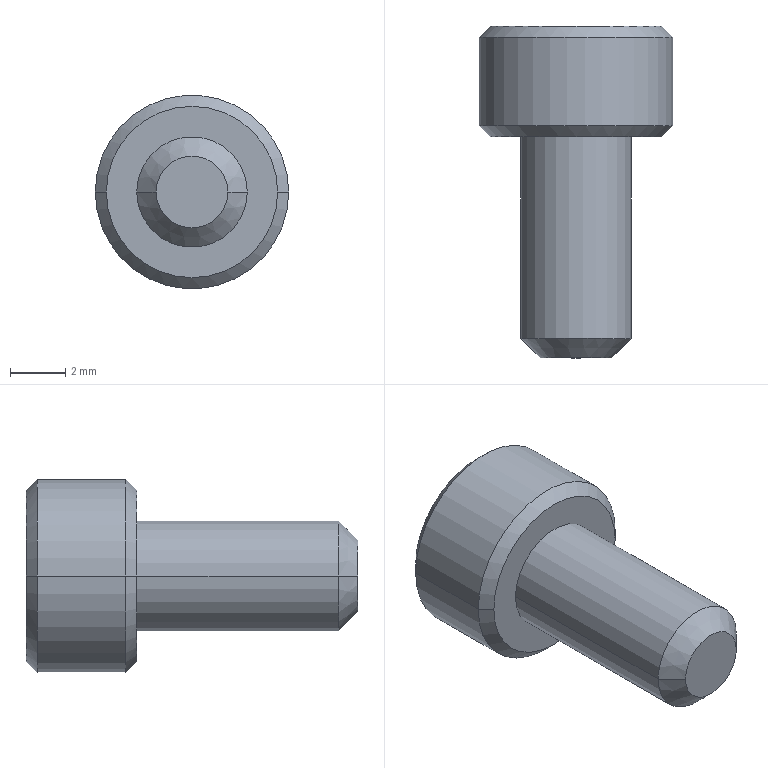Part | STEP file | BB62-M4-8L-1 | 1 solid | 27 faces | box 7 x 12 x 7 mm | volume 229.916 mm3 | plane 15 | cone 8 | cylinder 4 | commonest cylinder face diameters 4 x2 7 x2
STEP:
#1=CARTESIAN_POINT('',(0.,1.007,0.));
#2=VERTEX_POINT('',#1);
#3=CARTESIAN_POINT('',(1.72,2.,0.));
#4=VERTEX_POINT('',#3);
#5=CARTESIAN_POINT('',(0.,1.007,0.));
#6=DIRECTION('',(0.866,0.5,0.));
#7=VECTOR('',#6,1000.);
#8=LINE('',#5,#7);
#9=EDGE_CURVE('',#2,#4,#8,.T.);
#10=ORIENTED_EDGE('',*,*,#9,.F.);
#11=CARTESIAN_POINT('',(-1.72,2.,0.));
#12=VERTEX_POINT('',#11);
#13=CARTESIAN_POINT('',(0.,1.007,0.));
#14=DIRECTION('',(-0.866,0.5,0.));
#15=VECTOR('',#14,1000.);
#16=LINE('',#13,#15);
#17=EDGE_CURVE('',#2,#12,#16,.T.);
#18=ORIENTED_EDGE('',*,*,#17,.T.);
#19=CARTESIAN_POINT('',(-1.49,2.,0.86));
#20=VERTEX_POINT('',#19);
#21=CARTESIAN_POINT('',(0.,2.,0.));
#22=DIRECTION('',(0.,-1.,0.));
#23=DIRECTION('',(-1.,0.,0.));
#24=AXIS2_PLACEMENT_3D('',#21,#22,#23);
#25=CIRCLE('',#24,1.72);
#26=EDGE_CURVE('',#20,#12,#25,.T.);
#27=ORIENTED_EDGE('',*,*,#26,.F.);
#28=CARTESIAN_POINT('',(0.,2.,1.72));
#29=VERTEX_POINT('',#28);
#30=CARTESIAN_POINT('',(0.,2.,0.));
#31=DIRECTION('',(0.,-1.,0.));
#32=DIRECTION('',(-1.,0.,0.));
#33=AXIS2_PLACEMENT_3D('',#30,#31,#32);
#34=CIRCLE('',#33,1.72);
#35=EDGE_CURVE('',#29,#20,#34,.T.);
#36=ORIENTED_EDGE('',*,*,#35,.F.);
#37=CARTESIAN_POINT('',(1.49,2.,0.86));
#38=VERTEX_POINT('',#37);
#39=CARTESIAN_POINT('',(0.,2.,0.));
#40=DIRECTION('',(0.,-1.,0.));
#41=DIRECTION('',(-1.,0.,0.));
#42=AXIS2_PLACEMENT_3D('',#39,#40,#41);
#43=CIRCLE('',#42,1.72);
#44=EDGE_CURVE('',#38,#29,#43,.T.);
#45=ORIENTED_EDGE('',*,*,#44,.F.);
#46=CARTESIAN_POINT('',(0.,2.,0.));
#47=DIRECTION('',(0.,-1.,0.));
#48=DIRECTION('',(-1.,0.,0.));
#49=AXIS2_PLACEMENT_3D('',#46,#47,#48);
#50=CIRCLE('',#49,1.72);
#51=EDGE_CURVE('',#4,#38,#50,.T.);
#52=ORIENTED_EDGE('',*,*,#51,.F.);
#53=EDGE_LOOP('',(#10,#18,#27,#36,#45,#52));
#54=FACE_OUTER_BOUND('',#53,.T.);
#55=CARTESIAN_POINT('',(0.,1001.007,0.));
#56=DIRECTION('',(0.,1.,0.));
#57=DIRECTION('',(1.,0.,0.));
#58=AXIS2_PLACEMENT_3D('',#55,#56,#57);
#59=CONICAL_SURFACE('',#58,1732.051,1.047);
#60=ADVANCED_FACE('',(#54),#59,.F.);
#61=CARTESIAN_POINT('',(1.3,-8.,0.));
#62=VERTEX_POINT('',#61);
#63=CARTESIAN_POINT('',(-1.3,-8.,0.));
#64=VERTEX_POINT('',#63);
#65=CARTESIAN_POINT('',(0.,-8.,0.));
#66=DIRECTION('',(0.,1.,0.));
#67=DIRECTION('',(1.,0.,0.));
#68=AXIS2_PLACEMENT_3D('',#65,#66,#67);
#69=CIRCLE('',#68,1.3);
#70=EDGE_CURVE('',#62,#64,#69,.T.);
#71=ORIENTED_EDGE('',*,*,#70,.T.);
#72=CARTESIAN_POINT('',(-2.,-7.3,0.));
#73=VERTEX_POINT('',#72);
#74=CARTESIAN_POINT('',(-1.3,-8.,0.));
#75=DIRECTION('',(-0.7071,0.7071,0.));
#76=VECTOR('',#75,1000.);
#77=LINE('',#74,#76);
#78=EDGE_CURVE('',#64,#73,#77,.T.);
#79=ORIENTED_EDGE('',*,*,#78,.T.);
#80=CARTESIAN_POINT('',(2.,-7.3,0.));
#81=VERTEX_POINT('',#80);
#82=CARTESIAN_POINT('',(0.,-7.3,0.));
#83=DIRECTION('',(0.,-1.,0.));
#84=DIRECTION('',(-1.,0.,0.));
#85=AXIS2_PLACEMENT_3D('',#82,#83,#84);
#86=CIRCLE('',#85,2.);
#87=EDGE_CURVE('',#73,#81,#86,.T.);
#88=ORIENTED_EDGE('',*,*,#87,.T.);
#89=CARTESIAN_POINT('',(1.3,-8.,0.));
#90=DIRECTION('',(0.7071,0.7071,0.));
#91=VECTOR('',#90,1000.);
#92=LINE('',#89,#91);
#93=EDGE_CURVE('',#62,#81,#92,.T.);
#94=ORIENTED_EDGE('',*,*,#93,.F.);
#95=EDGE_LOOP('',(#71,#79,#88,#94));
#96=FACE_OUTER_BOUND('',#95,.T.);
#97=CARTESIAN_POINT('',(0.,-8.,0.));
#98=DIRECTION('',(0.,1.,0.));
#99=DIRECTION('',(1.,0.,0.));
#100=AXIS2_PLACEMENT_3D('',#97,#98,#99);
#101=CONICAL_SURFACE('',#100,1.3,0.7854);
#102=ADVANCED_FACE('',(#96),#101,.T.);
#103=ORIENTED_EDGE('',*,*,#87,.F.);
#104=CARTESIAN_POINT('',(-2.,0.,0.));
#105=VERTEX_POINT('',#104);
#106=CARTESIAN_POINT('',(-2.,-7.3,0.));
#107=DIRECTION('',(0.,1.,0.));
#108=VECTOR('',#107,1000.);
#109=LINE('',#106,#108);
#110=EDGE_CURVE('',#73,#105,#109,.T.);
#111=ORIENTED_EDGE('',*,*,#110,.T.);
#112=CARTESIAN_POINT('',(2.,0.,0.));
#113=VERTEX_POINT('',#112);
#114=CARTESIAN_POINT('',(0.,0.,0.));
#115=DIRECTION('',(0.,-1.,0.));
#116=DIRECTION('',(-1.,0.,0.));
#117=AXIS2_PLACEMENT_3D('',#114,#115,#116);
#118=CIRCLE('',#117,2.);
#119=EDGE_CURVE('',#105,#113,#118,.T.);
#120=ORIENTED_EDGE('',*,*,#119,.T.);
#121=CARTESIAN_POINT('',(2.,-7.3,0.));
#122=DIRECTION('',(0.,1.,0.));
#123=VECTOR('',#122,1000.);
#124=LINE('',#121,#123);
#125=EDGE_CURVE('',#81,#113,#124,.T.);
#126=ORIENTED_EDGE('',*,*,#125,.F.);
#127=EDGE_LOOP('',(#103,#111,#120,#126));
#128=FACE_OUTER_BOUND('',#127,.T.);
#129=CARTESIAN_POINT('',(0.,-7.3,0.));
#130=DIRECTION('',(0.,1.,0.));
#131=DIRECTION('',(1.,0.,0.));
#132=AXIS2_PLACEMENT_3D('',#129,#130,#131);
#133=CYLINDRICAL_SURFACE('',#132,2.);
#134=ADVANCED_FACE('',(#128),#133,.T.);
#135=CARTESIAN_POINT('',(-3.1,4.,0.));
#136=VERTEX_POINT('',#135);
#137=CARTESIAN_POINT('',(3.1,4.,0.));
#138=VERTEX_POINT('',#137);
#139=CARTESIAN_POINT('',(0.,4.,0.));
#140=DIRECTION('',(0.,-1.,0.));
#141=DIRECTION('',(-1.,0.,0.));
#142=AXIS2_PLACEMENT_3D('',#139,#140,#141);
#143=CIRCLE('',#142,3.1);
#144=EDGE_CURVE('',#136,#138,#143,.T.);
#145=ORIENTED_EDGE('',*,*,#144,.T.);
#146=CARTESIAN_POINT('',(3.5,3.6,0.));
#147=VERTEX_POINT('',#146);
#148=CARTESIAN_POINT('',(3.5,3.6,0.));
#149=DIRECTION('',(0.7071,-0.7071,0.));
#150=VECTOR('',#149,1000.);
#151=LINE('',#148,#150);
#152=EDGE_CURVE('',#138,#147,#151,.T.);
#153=ORIENTED_EDGE('',*,*,#152,.T.);
#154=CARTESIAN_POINT('',(-3.5,3.6,0.));
#155=VERTEX_POINT('',#154);
#156=CARTESIAN_POINT('',(0.,3.6,0.));
#157=DIRECTION('',(0.,-1.,0.));
#158=DIRECTION('',(-1.,0.,0.));
#159=AXIS2_PLACEMENT_3D('',#156,#157,#158);
#160=CIRCLE('',#159,3.5);
#161=EDGE_CURVE('',#155,#147,#160,.T.);
#162=ORIENTED_EDGE('',*,*,#161,.F.);
#163=CARTESIAN_POINT('',(-3.5,3.6,0.));
#164=DIRECTION('',(-0.7071,-0.7071,0.));
#165=VECTOR('',#164,1000.);
#166=LINE('',#163,#165);
#167=EDGE_CURVE('',#136,#155,#166,.T.);
#168=ORIENTED_EDGE('',*,*,#167,.F.);
#169=EDGE_LOOP('',(#145,#153,#162,#168));
#170=FACE_OUTER_BOUND('',#169,.T.);
#171=CARTESIAN_POINT('',(0.,3.6,0.));
#172=DIRECTION('',(0.,-1.,0.));
#173=DIRECTION('',(-1.,0.,0.));
#174=AXIS2_PLACEMENT_3D('',#171,#172,#173);
#175=CONICAL_SURFACE('',#174,3.5,0.7854);
#176=ADVANCED_FACE('',(#170),#175,.T.);
#177=ORIENTED_EDGE('',*,*,#161,.T.);
#178=CARTESIAN_POINT('',(3.5,0.4,0.));
#179=VERTEX_POINT('',#178);
#180=CARTESIAN_POINT('',(3.5,1.62,0.));
#181=DIRECTION('',(0.,-1.,0.));
#182=VECTOR('',#181,1000.);
#183=LINE('',#180,#182);
#184=EDGE_CURVE('',#147,#179,#183,.T.);
#185=ORIENTED_EDGE('',*,*,#184,.T.);
#186=CARTESIAN_POINT('',(-3.5,0.4,0.));
#187=VERTEX_POINT('',#186);
#188=CARTESIAN_POINT('',(0.,0.4,0.));
#189=DIRECTION('',(0.,-1.,0.));
#190=DIRECTION('',(-1.,0.,0.));
#191=AXIS2_PLACEMENT_3D('',#188,#189,#190);
#192=CIRCLE('',#191,3.5);
#193=EDGE_CURVE('',#187,#179,#192,.T.);
#194=ORIENTED_EDGE('',*,*,#193,.F.);
#195=CARTESIAN_POINT('',(-3.5,1.62,0.));
#196=DIRECTION('',(0.,-1.,0.));
#197=VECTOR('',#196,1000.);
#198=LINE('',#195,#197);
#199=EDGE_CURVE('',#155,#187,#198,.T.);
#200=ORIENTED_EDGE('',*,*,#199,.F.);
#201=EDGE_LOOP('',(#177,#185,#194,#200));
#202=FACE_OUTER_BOUND('',#201,.T.);
#203=CARTESIAN_POINT('',(0.,1.62,0.));
#204=DIRECTION('',(0.,-1.,0.));
#205=DIRECTION('',(-1.,0.,0.));
#206=AXIS2_PLACEMENT_3D('',#203,#204,#205);
#207=CYLINDRICAL_SURFACE('',#206,3.5);
#208=ADVANCED_FACE('',(#202),#207,.T.);
#209=CARTESIAN_POINT('',(-3.1,0.,0.));
#210=VERTEX_POINT('',#209);
#211=CARTESIAN_POINT('',(3.1,0.,0.));
#212=VERTEX_POINT('',#211);
#213=CARTESIAN_POINT('',(0.,0.,0.));
#214=DIRECTION('',(0.,-1.,0.));
#215=DIRECTION('',(-1.,0.,0.));
#216=AXIS2_PLACEMENT_3D('',#213,#214,#215);
#217=CIRCLE('',#216,3.1);
#218=EDGE_CURVE('',#210,#212,#217,.T.);
#219=ORIENTED_EDGE('',*,*,#218,.F.);
#220=CARTESIAN_POINT('',(-3.1,0.,0.));
#221=DIRECTION('',(-0.7071,0.7071,0.));
#222=VECTOR('',#221,1000.);
#223=LINE('',#220,#222);
#224=EDGE_CURVE('',#210,#187,#223,.T.);
#225=ORIENTED_EDGE('',*,*,#224,.T.);
#226=ORIENTED_EDGE('',*,*,#193,.T.);
#227=CARTESIAN_POINT('',(3.1,0.,0.));
#228=DIRECTION('',(0.7071,0.7071,0.));
#229=VECTOR('',#228,1000.);
#230=LINE('',#227,#229);
#231=EDGE_CURVE('',#212,#179,#230,.T.);
#232=ORIENTED_EDGE('',*,*,#231,.F.);
#233=EDGE_LOOP('',(#219,#225,#226,#232));
#234=FACE_OUTER_BOUND('',#233,.T.);
#235=CARTESIAN_POINT('',(0.,0.,0.));
#236=DIRECTION('',(0.,1.,0.));
#237=DIRECTION('',(1.,0.,0.));
#238=AXIS2_PLACEMENT_3D('',#235,#236,#237);
#239=CONICAL_SURFACE('',#238,3.1,0.7854);
#240=ADVANCED_FACE('',(#234),#239,.T.);
#241=ORIENTED_EDGE('',*,*,#144,.F.);
#242=CARTESIAN_POINT('',(0.,4.,0.));
#243=DIRECTION('',(0.,-1.,0.));
#244=DIRECTION('',(-1.,0.,0.));
#245=AXIS2_PLACEMENT_3D('',#242,#243,#244);
#246=CIRCLE('',#245,3.1);
#247=EDGE_CURVE('',#138,#136,#246,.T.);
#248=ORIENTED_EDGE('',*,*,#247,.F.);
#249=EDGE_LOOP('',(#241,#248));
#250=FACE_OUTER_BOUND('',#249,.T.);
#251=CARTESIAN_POINT('',(0.,4.,-1.72));
#252=VERTEX_POINT('',#251);
#253=CARTESIAN_POINT('',(-1.49,4.,-0.86));
#254=VERTEX_POINT('',#253);
#255=CARTESIAN_POINT('',(0.,4.,-1.72));
#256=DIRECTION('',(-0.866,0.,0.5));
#257=VECTOR('',#256,1000.);
#258=LINE('',#255,#257);
#259=EDGE_CURVE('',#252,#254,#258,.T.);
#260=ORIENTED_EDGE('',*,*,#259,.F.);
#261=CARTESIAN_POINT('',(1.49,4.,-0.86));
#262=VERTEX_POINT('',#261);
#263=CARTESIAN_POINT('',(1.49,4.,-0.86));
#264=DIRECTION('',(-0.866,0.,-0.5));
#265=VECTOR('',#264,1000.);
#266=LINE('',#263,#265);
#267=EDGE_CURVE('',#262,#252,#266,.T.);
#268=ORIENTED_EDGE('',*,*,#267,.F.);
#269=CARTESIAN_POINT('',(1.49,4.,0.86));
#270=VERTEX_POINT('',#269);
#271=CARTESIAN_POINT('',(1.49,4.,0.86));
#272=DIRECTION('',(0.,0.,-1.));
#273=VECTOR('',#272,1000.);
#274=LINE('',#271,#273);
#275=EDGE_CURVE('',#270,#262,#274,.T.);
#276=ORIENTED_EDGE('',*,*,#275,.F.);
#277=CARTESIAN_POINT('',(0.,4.,1.72));
#278=VERTEX_POINT('',#277);
#279=CARTESIAN_POINT('',(0.,4.,1.72));
#280=DIRECTION('',(0.866,0.,-0.5));
#281=VECTOR('',#280,1000.);
#282=LINE('',#279,#281);
#283=EDGE_CURVE('',#278,#270,#282,.T.);
#284=ORIENTED_EDGE('',*,*,#283,.F.);
#285=CARTESIAN_POINT('',(-1.49,4.,0.86));
#286=VERTEX_POINT('',#285);
#287=CARTESIAN_POINT('',(-1.49,4.,0.86));
#288=DIRECTION('',(0.866,0.,0.5));
#289=VECTOR('',#288,1000.);
#290=LINE('',#287,#289);
#291=EDGE_CURVE('',#286,#278,#290,.T.);
#292=ORIENTED_EDGE('',*,*,#291,.F.);
#293=CARTESIAN_POINT('',(-1.49,4.,-0.86));
#294=DIRECTION('',(0.,0.,1.));
#295=VECTOR('',#294,1000.);
#296=LINE('',#293,#295);
#297=EDGE_CURVE('',#254,#286,#296,.T.);
#298=ORIENTED_EDGE('',*,*,#297,.F.);
#299=EDGE_LOOP('',(#260,#268,#276,#284,#292,#298));
#300=FACE_BOUND('',#299,.T.);
#301=CARTESIAN_POINT('',(3.1,4.,0.));
#302=DIRECTION('',(0.,1.,0.));
#303=DIRECTION('',(1.,0.,0.));
#304=AXIS2_PLACEMENT_3D('',#301,#302,#303);
#305=PLANE('',#304);
#306=ADVANCED_FACE('',(#250,#300),#305,.T.);
#307=CARTESIAN_POINT('',(0.,0.,0.));
#308=DIRECTION('',(0.,-1.,0.));
#309=DIRECTION('',(-1.,0.,0.));
#310=AXIS2_PLACEMENT_3D('',#307,#308,#309);
#311=CIRCLE('',#310,2.);
#312=EDGE_CURVE('',#113,#105,#311,.T.);
#313=ORIENTED_EDGE('',*,*,#312,.F.);
#314=ORIENTED_EDGE('',*,*,#119,.F.);
#315=EDGE_LOOP('',(#313,#314));
#316=FACE_BOUND('',#315,.T.);
#317=CARTESIAN_POINT('',(0.,0.,0.));
#318=DIRECTION('',(0.,-1.,0.));
#319=DIRECTION('',(-1.,0.,0.));
#320=AXIS2_PLACEMENT_3D('',#317,#318,#319);
#321=CIRCLE('',#320,3.1);
#322=EDGE_CURVE('',#212,#210,#321,.T.);
#323=ORIENTED_EDGE('',*,*,#322,.T.);
#324=ORIENTED_EDGE('',*,*,#218,.T.);
#325=EDGE_LOOP('',(#323,#324));
#326=FACE_OUTER_BOUND('',#325,.T.);
#327=CARTESIAN_POINT('',(0.,0.,0.));
#328=DIRECTION('',(0.,-1.,0.));
#329=DIRECTION('',(-1.,0.,0.));
#330=AXIS2_PLACEMENT_3D('',#327,#328,#329);
#331=PLANE('',#330);
#332=ADVANCED_FACE('',(#316,#326),#331,.T.);
#333=ORIENTED_EDGE('',*,*,#224,.F.);
#334=ORIENTED_EDGE('',*,*,#322,.F.);
#335=ORIENTED_EDGE('',*,*,#231,.T.);
#336=CARTESIAN_POINT('',(0.,0.4,0.));
#337=DIRECTION('',(0.,-1.,0.));
#338=DIRECTION('',(-1.,0.,0.));
#339=AXIS2_PLACEMENT_3D('',#336,#337,#338);
#340=CIRCLE('',#339,3.5);
#341=EDGE_CURVE('',#179,#187,#340,.T.);
#342=ORIENTED_EDGE('',*,*,#341,.T.);
#343=EDGE_LOOP('',(#333,#334,#335,#342));
#344=FACE_OUTER_BOUND('',#343,.T.);
#345=CARTESIAN_POINT('',(0.,0.,0.));
#346=DIRECTION('',(0.,1.,0.));
#347=DIRECTION('',(1.,0.,0.));
#348=AXIS2_PLACEMENT_3D('',#345,#346,#347);
#349=CONICAL_SURFACE('',#348,3.1,0.7854);
#350=ADVANCED_FACE('',(#344),#349,.T.);
#351=ORIENTED_EDGE('',*,*,#184,.F.);
#352=CARTESIAN_POINT('',(0.,3.6,0.));
#353=DIRECTION('',(0.,-1.,0.));
#354=DIRECTION('',(-1.,0.,0.));
#355=AXIS2_PLACEMENT_3D('',#352,#353,#354);
#356=CIRCLE('',#355,3.5);
#357=EDGE_CURVE('',#147,#155,#356,.T.);
#358=ORIENTED_EDGE('',*,*,#357,.T.);
#359=ORIENTED_EDGE('',*,*,#199,.T.);
#360=ORIENTED_EDGE('',*,*,#341,.F.);
#361=EDGE_LOOP('',(#351,#358,#359,#360));
#362=FACE_OUTER_BOUND('',#361,.T.);
#363=CARTESIAN_POINT('',(0.,1.62,0.));
#364=DIRECTION('',(0.,-1.,0.));
#365=DIRECTION('',(-1.,0.,0.));
#366=AXIS2_PLACEMENT_3D('',#363,#364,#365);
#367=CYLINDRICAL_SURFACE('',#366,3.5);
#368=ADVANCED_FACE('',(#362),#367,.T.);
#369=ORIENTED_EDGE('',*,*,#152,.F.);
#370=ORIENTED_EDGE('',*,*,#247,.T.);
#371=ORIENTED_EDGE('',*,*,#167,.T.);
#372=ORIENTED_EDGE('',*,*,#357,.F.);
#373=EDGE_LOOP('',(#369,#370,#371,#372));
#374=FACE_OUTER_BOUND('',#373,.T.);
#375=CARTESIAN_POINT('',(0.,3.6,0.));
#376=DIRECTION('',(0.,-1.,0.));
#377=DIRECTION('',(-1.,0.,0.));
#378=AXIS2_PLACEMENT_3D('',#375,#376,#377);
#379=CONICAL_SURFACE('',#378,3.5,0.7854);
#380=ADVANCED_FACE('',(#374),#379,.T.);
#381=ORIENTED_EDGE('',*,*,#110,.F.);
#382=CARTESIAN_POINT('',(0.,-7.3,0.));
#383=DIRECTION('',(0.,-1.,0.));
#384=DIRECTION('',(-1.,0.,0.));
#385=AXIS2_PLACEMENT_3D('',#382,#383,#384);
#386=CIRCLE('',#385,2.);
#387=EDGE_CURVE('',#81,#73,#386,.T.);
#388=ORIENTED_EDGE('',*,*,#387,.F.);
#389=ORIENTED_EDGE('',*,*,#125,.T.);
#390=ORIENTED_EDGE('',*,*,#312,.T.);
#391=EDGE_LOOP('',(#381,#388,#389,#390));
#392=FACE_OUTER_BOUND('',#391,.T.);
#393=CARTESIAN_POINT('',(0.,-7.3,0.));
#394=DIRECTION('',(0.,1.,0.));
#395=DIRECTION('',(1.,0.,0.));
#396=AXIS2_PLACEMENT_3D('',#393,#394,#395);
#397=CYLINDRICAL_SURFACE('',#396,2.);
#398=ADVANCED_FACE('',(#392),#397,.T.);
#399=ORIENTED_EDGE('',*,*,#70,.F.);
#400=CARTESIAN_POINT('',(0.,-8.,0.));
#401=DIRECTION('',(0.,1.,0.));
#402=DIRECTION('',(1.,0.,0.));
#403=AXIS2_PLACEMENT_3D('',#400,#401,#402);
#404=CIRCLE('',#403,1.3);
#405=EDGE_CURVE('',#64,#62,#404,.T.);
#406=ORIENTED_EDGE('',*,*,#405,.F.);
#407=EDGE_LOOP('',(#399,#406));
#408=FACE_OUTER_BOUND('',#407,.T.);
#409=CARTESIAN_POINT('',(0.,-8.,0.));
#410=DIRECTION('',(0.,-1.,0.));
#411=DIRECTION('',(-1.,0.,0.));
#412=AXIS2_PLACEMENT_3D('',#409,#410,#411);
#413=PLANE('',#412);
#414=ADVANCED_FACE('',(#408),#413,.T.);
#415=ORIENTED_EDGE('',*,*,#78,.F.);
#416=ORIENTED_EDGE('',*,*,#405,.T.);
#417=ORIENTED_EDGE('',*,*,#93,.T.);
#418=ORIENTED_EDGE('',*,*,#387,.T.);
#419=EDGE_LOOP('',(#415,#416,#417,#418));
#420=FACE_OUTER_BOUND('',#419,.T.);
#421=CARTESIAN_POINT('',(0.,-8.,0.));
#422=DIRECTION('',(0.,1.,0.));
#423=DIRECTION('',(1.,0.,0.));
#424=AXIS2_PLACEMENT_3D('',#421,#422,#423);
#425=CONICAL_SURFACE('',#424,1.3,0.7854);
#426=ADVANCED_FACE('',(#420),#425,.T.);
#427=CARTESIAN_POINT('',(1.49,2.,-0.86));
#428=VERTEX_POINT('',#427);
#429=CARTESIAN_POINT('',(0.,2.,-1.72));
#430=VERTEX_POINT('',#429);
#431=CARTESIAN_POINT('',(1.49,2.,-0.86));
#432=DIRECTION('',(-0.866,0.,-0.5));
#433=VECTOR('',#432,1000.);
#434=LINE('',#431,#433);
#435=EDGE_CURVE('',#428,#430,#434,.T.);
#436=ORIENTED_EDGE('',*,*,#435,.F.);
#437=CARTESIAN_POINT('',(1.49,4.,-0.86));
#438=DIRECTION('',(0.,-1.,0.));
#439=VECTOR('',#438,1000.);
#440=LINE('',#437,#439);
#441=EDGE_CURVE('',#262,#428,#440,.T.);
#442=ORIENTED_EDGE('',*,*,#441,.F.);
#443=ORIENTED_EDGE('',*,*,#267,.T.);
#444=CARTESIAN_POINT('',(0.,4.,-1.72));
#445=DIRECTION('',(0.,-1.,0.));
#446=VECTOR('',#445,1000.);
#447=LINE('',#444,#446);
#448=EDGE_CURVE('',#252,#430,#447,.T.);
#449=ORIENTED_EDGE('',*,*,#448,.T.);
#450=EDGE_LOOP('',(#436,#442,#443,#449));
#451=FACE_OUTER_BOUND('',#450,.T.);
#452=CARTESIAN_POINT('',(1.49,4.,-0.86));
#453=DIRECTION('',(-0.5,0.,0.866));
#454=DIRECTION('',(0.866,0.,0.5));
#455=AXIS2_PLACEMENT_3D('',#452,#453,#454);
#456=PLANE('',#455);
#457=ADVANCED_FACE('',(#451),#456,.T.);
#458=CARTESIAN_POINT('',(-1.49,2.,-0.86));
#459=VERTEX_POINT('',#458);
#460=CARTESIAN_POINT('',(0.,2.,-1.72));
#461=DIRECTION('',(-0.866,0.,0.5));
#462=VECTOR('',#461,1000.);
#463=LINE('',#460,#462);
#464=EDGE_CURVE('',#430,#459,#463,.T.);
#465=ORIENTED_EDGE('',*,*,#464,.F.);
#466=ORIENTED_EDGE('',*,*,#448,.F.);
#467=ORIENTED_EDGE('',*,*,#259,.T.);
#468=CARTESIAN_POINT('',(-1.49,4.,-0.86));
#469=DIRECTION('',(0.,-1.,0.));
#470=VECTOR('',#469,1000.);
#471=LINE('',#468,#470);
#472=EDGE_CURVE('',#254,#459,#471,.T.);
#473=ORIENTED_EDGE('',*,*,#472,.T.);
#474=EDGE_LOOP('',(#465,#466,#467,#473));
#475=FACE_OUTER_BOUND('',#474,.T.);
#476=CARTESIAN_POINT('',(0.,4.,-1.72));
#477=DIRECTION('',(0.5,0.,0.866));
#478=DIRECTION('',(0.866,0.,-0.5));
#479=AXIS2_PLACEMENT_3D('',#476,#477,#478);
#480=PLANE('',#479);
#481=ADVANCED_FACE('',(#475),#480,.T.);
#482=CARTESIAN_POINT('',(-1.49,2.,-0.86));
#483=DIRECTION('',(0.,0.,1.));
#484=VECTOR('',#483,1000.);
#485=LINE('',#482,#484);
#486=EDGE_CURVE('',#459,#20,#485,.T.);
#487=ORIENTED_EDGE('',*,*,#486,.F.);
#488=ORIENTED_EDGE('',*,*,#472,.F.);
#489=ORIENTED_EDGE('',*,*,#297,.T.);
#490=CARTESIAN_POINT('',(-1.49,4.,0.86));
#491=DIRECTION('',(0.,-1.,0.));
#492=VECTOR('',#491,1000.);
#493=LINE('',#490,#492);
#494=EDGE_CURVE('',#286,#20,#493,.T.);
#495=ORIENTED_EDGE('',*,*,#494,.T.);
#496=EDGE_LOOP('',(#487,#488,#489,#495));
#497=FACE_OUTER_BOUND('',#496,.T.);
#498=CARTESIAN_POINT('',(-1.49,4.,-0.86));
#499=DIRECTION('',(1.,0.,0.));
#500=DIRECTION('',(0.,0.,-1.));
#501=AXIS2_PLACEMENT_3D('',#498,#499,#500);
#502=PLANE('',#501);
#503=ADVANCED_FACE('',(#497),#502,.T.);
#504=CARTESIAN_POINT('',(-1.49,2.,0.86));
#505=DIRECTION('',(0.866,0.,0.5));
#506=VECTOR('',#505,1000.);
#507=LINE('',#504,#506);
#508=EDGE_CURVE('',#20,#29,#507,.T.);
#509=ORIENTED_EDGE('',*,*,#508,.F.);
#510=ORIENTED_EDGE('',*,*,#494,.F.);
#511=ORIENTED_EDGE('',*,*,#291,.T.);
#512=CARTESIAN_POINT('',(0.,4.,1.72));
#513=DIRECTION('',(0.,-1.,0.));
#514=VECTOR('',#513,1000.);
#515=LINE('',#512,#514);
#516=EDGE_CURVE('',#278,#29,#515,.T.);
#517=ORIENTED_EDGE('',*,*,#516,.T.);
#518=EDGE_LOOP('',(#509,#510,#511,#517));
#519=FACE_OUTER_BOUND('',#518,.T.);
#520=CARTESIAN_POINT('',(-1.49,4.,0.86));
#521=DIRECTION('',(0.5,0.,-0.866));
#522=DIRECTION('',(-0.866,0.,-0.5));
#523=AXIS2_PLACEMENT_3D('',#520,#521,#522);
#524=PLANE('',#523);
#525=ADVANCED_FACE('',(#519),#524,.T.);
#526=CARTESIAN_POINT('',(0.,2.,1.72));
#527=DIRECTION('',(0.866,0.,-0.5));
#528=VECTOR('',#527,1000.);
#529=LINE('',#526,#528);
#530=EDGE_CURVE('',#29,#38,#529,.T.);
#531=ORIENTED_EDGE('',*,*,#530,.F.);
#532=ORIENTED_EDGE('',*,*,#516,.F.);
#533=ORIENTED_EDGE('',*,*,#283,.T.);
#534=CARTESIAN_POINT('',(1.49,4.,0.86));
#535=DIRECTION('',(0.,-1.,0.));
#536=VECTOR('',#535,1000.);
#537=LINE('',#534,#536);
#538=EDGE_CURVE('',#270,#38,#537,.T.);
#539=ORIENTED_EDGE('',*,*,#538,.T.);
#540=EDGE_LOOP('',(#531,#532,#533,#539));
#541=FACE_OUTER_BOUND('',#540,.T.);
#542=CARTESIAN_POINT('',(0.,4.,1.72));
#543=DIRECTION('',(-0.5,0.,-0.866));
#544=DIRECTION('',(-0.866,0.,0.5));
#545=AXIS2_PLACEMENT_3D('',#542,#543,#544);
#546=PLANE('',#545);
#547=ADVANCED_FACE('',(#541),#546,.T.);
#548=CARTESIAN_POINT('',(1.49,2.,0.86));
#549=DIRECTION('',(0.,0.,-1.));
#550=VECTOR('',#549,1000.);
#551=LINE('',#548,#550);
#552=EDGE_CURVE('',#38,#428,#551,.T.);
#553=ORIENTED_EDGE('',*,*,#552,.F.);
#554=ORIENTED_EDGE('',*,*,#538,.F.);
#555=ORIENTED_EDGE('',*,*,#275,.T.);
#556=ORIENTED_EDGE('',*,*,#441,.T.);
#557=EDGE_LOOP('',(#553,#554,#555,#556));
#558=FACE_OUTER_BOUND('',#557,.T.);
#559=CARTESIAN_POINT('',(1.49,4.,0.86));
#560=DIRECTION('',(-1.,0.,0.));
#561=DIRECTION('',(0.,0.,1.));
#562=AXIS2_PLACEMENT_3D('',#559,#560,#561);
#563=PLANE('',#562);
#564=ADVANCED_FACE('',(#558),#563,.T.);
#565=ORIENTED_EDGE('',*,*,#435,.T.);
#566=CARTESIAN_POINT('',(0.,2.,0.));
#567=DIRECTION('',(0.,-1.,0.));
#568=DIRECTION('',(-1.,0.,0.));
#569=AXIS2_PLACEMENT_3D('',#566,#567,#568);
#570=CIRCLE('',#569,1.72);
#571=EDGE_CURVE('',#430,#428,#570,.T.);
#572=ORIENTED_EDGE('',*,*,#571,.T.);
#573=EDGE_LOOP('',(#565,#572));
#574=FACE_OUTER_BOUND('',#573,.T.);
#575=CARTESIAN_POINT('',(0.,2.,0.));
#576=DIRECTION('',(0.,1.,0.));
#577=DIRECTION('',(1.,0.,0.));
#578=AXIS2_PLACEMENT_3D('',#575,#576,#577);
#579=PLANE('',#578);
#580=ADVANCED_FACE('',(#574),#579,.F.);
#581=ORIENTED_EDGE('',*,*,#552,.T.);
#582=CARTESIAN_POINT('',(0.,2.,0.));
#583=DIRECTION('',(0.,-1.,0.));
#584=DIRECTION('',(-1.,0.,0.));
#585=AXIS2_PLACEMENT_3D('',#582,#583,#584);
#586=CIRCLE('',#585,1.72);
#587=EDGE_CURVE('',#428,#4,#586,.T.);
#588=ORIENTED_EDGE('',*,*,#587,.T.);
#589=ORIENTED_EDGE('',*,*,#51,.T.);
#590=EDGE_LOOP('',(#581,#588,#589));
#591=FACE_OUTER_BOUND('',#590,.T.);
#592=CARTESIAN_POINT('',(0.,2.,0.));
#593=DIRECTION('',(0.,1.,0.));
#594=DIRECTION('',(1.,0.,0.));
#595=AXIS2_PLACEMENT_3D('',#592,#593,#594);
#596=PLANE('',#595);
#597=ADVANCED_FACE('',(#591),#596,.F.);
#598=ORIENTED_EDGE('',*,*,#530,.T.);
#599=ORIENTED_EDGE('',*,*,#44,.T.);
#600=EDGE_LOOP('',(#598,#599));
#601=FACE_OUTER_BOUND('',#600,.T.);
#602=CARTESIAN_POINT('',(0.,2.,0.));
#603=DIRECTION('',(0.,1.,0.));
#604=DIRECTION('',(1.,0.,0.));
#605=AXIS2_PLACEMENT_3D('',#602,#603,#604);
#606=PLANE('',#605);
#607=ADVANCED_FACE('',(#601),#606,.F.);
#608=ORIENTED_EDGE('',*,*,#508,.T.);
#609=ORIENTED_EDGE('',*,*,#35,.T.);
#610=EDGE_LOOP('',(#608,#609));
#611=FACE_OUTER_BOUND('',#610,.T.);
#612=CARTESIAN_POINT('',(0.,2.,0.));
#613=DIRECTION('',(0.,1.,0.));
#614=DIRECTION('',(1.,0.,0.));
#615=AXIS2_PLACEMENT_3D('',#612,#613,#614);
#616=PLANE('',#615);
#617=ADVANCED_FACE('',(#611),#616,.F.);
#618=ORIENTED_EDGE('',*,*,#486,.T.);
#619=ORIENTED_EDGE('',*,*,#26,.T.);
#620=CARTESIAN_POINT('',(0.,2.,0.));
#621=DIRECTION('',(0.,-1.,0.));
#622=DIRECTION('',(-1.,0.,0.));
#623=AXIS2_PLACEMENT_3D('',#620,#621,#622);
#624=CIRCLE('',#623,1.72);
#625=EDGE_CURVE('',#12,#459,#624,.T.);
#626=ORIENTED_EDGE('',*,*,#625,.T.);
#627=EDGE_LOOP('',(#618,#619,#626));
#628=FACE_OUTER_BOUND('',#627,.T.);
#629=CARTESIAN_POINT('',(0.,2.,0.));
#630=DIRECTION('',(0.,1.,0.));
#631=DIRECTION('',(1.,0.,0.));
#632=AXIS2_PLACEMENT_3D('',#629,#630,#631);
#633=PLANE('',#632);
#634=ADVANCED_FACE('',(#628),#633,.F.);
#635=ORIENTED_EDGE('',*,*,#464,.T.);
#636=CARTESIAN_POINT('',(0.,2.,0.));
#637=DIRECTION('',(0.,-1.,0.));
#638=DIRECTION('',(-1.,0.,0.));
#639=AXIS2_PLACEMENT_3D('',#636,#637,#638);
#640=CIRCLE('',#639,1.72);
#641=EDGE_CURVE('',#459,#430,#640,.T.);
#642=ORIENTED_EDGE('',*,*,#641,.T.);
#643=EDGE_LOOP('',(#635,#642));
#644=FACE_OUTER_BOUND('',#643,.T.);
#645=CARTESIAN_POINT('',(0.,2.,0.));
#646=DIRECTION('',(0.,1.,0.));
#647=DIRECTION('',(1.,0.,0.));
#648=AXIS2_PLACEMENT_3D('',#645,#646,#647);
#649=PLANE('',#648);
#650=ADVANCED_FACE('',(#644),#649,.F.);
#651=ORIENTED_EDGE('',*,*,#17,.F.);
#652=ORIENTED_EDGE('',*,*,#9,.T.);
#653=ORIENTED_EDGE('',*,*,#587,.F.);
#654=ORIENTED_EDGE('',*,*,#571,.F.);
#655=ORIENTED_EDGE('',*,*,#641,.F.);
#656=ORIENTED_EDGE('',*,*,#625,.F.);
#657=EDGE_LOOP('',(#651,#652,#653,#654,#655,#656));
#658=FACE_OUTER_BOUND('',#657,.T.);
#659=CARTESIAN_POINT('',(0.,1001.007,0.));
#660=DIRECTION('',(0.,1.,0.));
#661=DIRECTION('',(1.,0.,0.));
#662=AXIS2_PLACEMENT_3D('',#659,#660,#661);
#663=CONICAL_SURFACE('',#662,1732.051,1.047);
#664=ADVANCED_FACE('',(#658),#663,.F.);
#665=CLOSED_SHELL('',(#60,#102,#134,#176,#208,#240,#306,#332,#350,#368,#380,#398,#414,#426,#457,#481,#503,#525,#547,#564,#580,#597,#607,#617,#634,#650,#664));
#666=MANIFOLD_SOLID_BREP('',#665);
#667=CARTESIAN_POINT('',(0.,0.,0.));
#668=DIRECTION('',(0.,0.,1.));
#669=DIRECTION('',(1.,0.,0.));
#670=AXIS2_PLACEMENT_3D('',#667,#668,#669);
#671=(LENGTH_UNIT()NAMED_UNIT(*)SI_UNIT(.MILLI.,.METRE.));
#672=UNCERTAINTY_MEASURE_WITH_UNIT(LENGTH_MEASURE(0.00001),#671,'','');
#673=(NAMED_UNIT(*)PLANE_ANGLE_UNIT()SI_UNIT($,.RADIAN.));
#674=(NAMED_UNIT(*)SI_UNIT($,.STERADIAN.)SOLID_ANGLE_UNIT());
#675=(GEOMETRIC_REPRESENTATION_CONTEXT(3)GLOBAL_UNCERTAINTY_ASSIGNED_CONTEXT((#672))GLOBAL_UNIT_ASSIGNED_CONTEXT((#671,#673,#674))REPRESENTATION_CONTEXT('',''));
#676=ADVANCED_BREP_SHAPE_REPRESENTATION('',(#666,#670),#675);